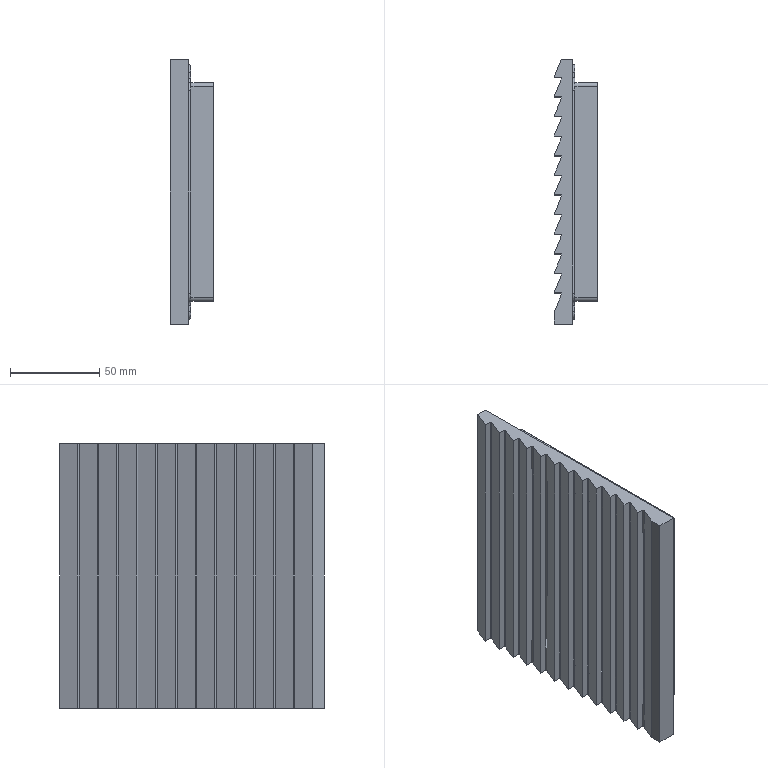Part | STEP file | FKL6622 cabinet fan and filter[FKL6622.230]_filter | 1 solid | 373 faces | box 24.5 x 148.5 x 148.5 mm | volume 148645 mm3 | plane 299 | spline 30 | cylinder 28 | torus 16 | commonest cylinder face diameters 2 x12 4.2 x8 0.4 x4 4 x4